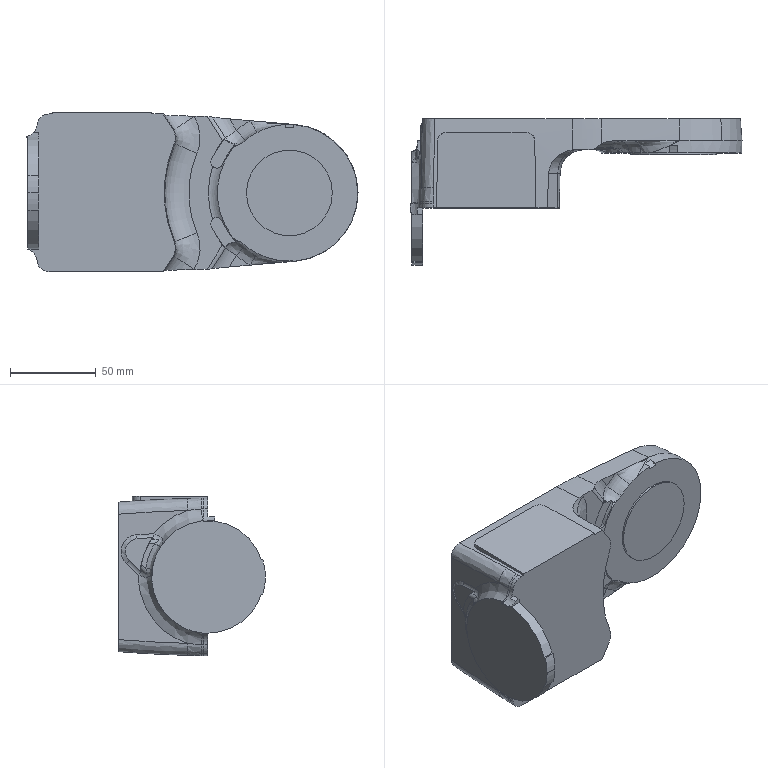Part | STEP file | ASND-0110-IRB120_3-58_IRC5_Link4_rev0 | 1 solid | 106 faces | box 193.368 x 85.5 x 92.955 mm | volume 549837 mm3 | cylinder 32 | spline 32 | plane 30 | cone 4 | other 4 | torus 4 | commonest cylinder face diameters 6 x4 1600 x4 7 x2 8 x2 10 x2 16 x2